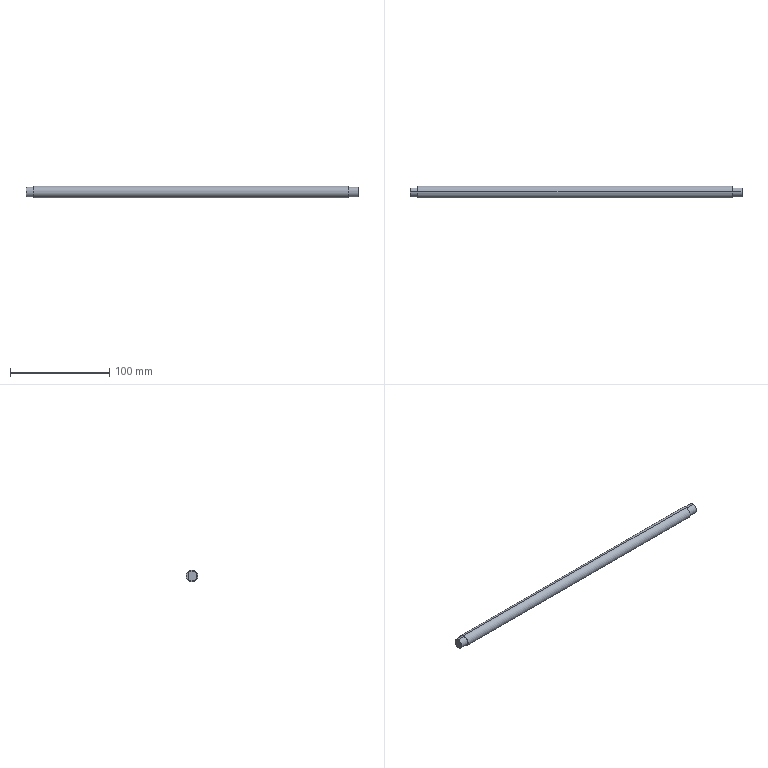Part | STEP file | 04-01 Φ12 chrome-plated rod | 1 solid | 14 faces | box 335 x 12 x 12 mm | volume 37192 mm3 | cylinder 8 | plane 6 | commonest cylinder face diameters 10 x6 12 x2
STEP:
#1=CARTESIAN_POINT('',(0.,0.,0.));
#2=DIRECTION('',(0.,0.,1.));
#3=DIRECTION('',(1.,0.,0.));
#4=AXIS2_PLACEMENT_3D('',#1,#2,#3);
#5=CARTESIAN_POINT('',(325.,0.,5.));
#6=VERTEX_POINT('',#5);
#7=CARTESIAN_POINT('',(325.,4.,3.));
#8=VERTEX_POINT('',#7);
#9=CARTESIAN_POINT('',(325.,0.,0.));
#10=DIRECTION('',(-1.,0.,0.));
#11=DIRECTION('',(0.,0.,-1.));
#12=AXIS2_PLACEMENT_3D('',#9,#10,#11);
#13=CIRCLE('',#12,5.);
#14=CARTESIAN_POINT('',(325.,0.,0.));
#15=DIRECTION('',(1.,0.,0.));
#16=DIRECTION('',(0.,0.,-1.));
#17=AXIS2_PLACEMENT_3D('',#14,#15,#16);
#18=CYLINDRICAL_SURFACE('',#17,5.);
#19=CARTESIAN_POINT('',(6.283,0.));
#20=DIRECTION('',(-1.,0.));
#21=VECTOR('',#20,1.);
#22=LINE('',#19,#21);
#23=(GEOMETRIC_REPRESENTATION_CONTEXT(2)PARAMETRIC_REPRESENTATION_CONTEXT()REPRESENTATION_CONTEXT('',''));
#24=DEFINITIONAL_REPRESENTATION('',(#22),#23);
#25=PCURVE('',#18,#24);
#26=CARTESIAN_POINT('',(325.,-6.072,6.072));
#27=DIRECTION('',(1.,0.,0.));
#28=DIRECTION('',(0.,0.,-1.));
#29=AXIS2_PLACEMENT_3D('',#26,#27,#28);
#30=PLANE('',#29);
#31=CARTESIAN_POINT('',(11.072,6.072));
#32=CARTESIAN_POINT('',(11.072,-2.588));
#33=CARTESIAN_POINT('',(3.572,1.742));
#34=CARTESIAN_POINT('',(-3.928,6.072));
#35=CARTESIAN_POINT('',(3.572,10.402));
#36=CARTESIAN_POINT('',(11.072,14.732));
#37=CARTESIAN_POINT('',(11.072,6.072));
#38=(BOUNDED_CURVE()B_SPLINE_CURVE(2,(#31,#32,#33,#34,#35,#36,#37),.UNSPECIFIED.,.T.,.F.)B_SPLINE_CURVE_WITH_KNOTS((1,2,2,2,2,1),(-2.094,0.,2.094,4.189,6.283,8.378),.UNSPECIFIED.)CURVE()GEOMETRIC_REPRESENTATION_ITEM()RATIONAL_B_SPLINE_CURVE((1.,0.5,1.,0.5,1.,0.5,1.))REPRESENTATION_ITEM(''));
#39=(GEOMETRIC_REPRESENTATION_CONTEXT(2)PARAMETRIC_REPRESENTATION_CONTEXT()REPRESENTATION_CONTEXT('',''));
#40=DEFINITIONAL_REPRESENTATION('',(#38),#39);
#41=PCURVE('',#30,#40);
#42=SURFACE_CURVE('',#13,(#25,#41),.PCURVE_S1.);
#43=EDGE_CURVE('',#6,#8,#42,.T.);
#44=ORIENTED_EDGE('',*,*,#43,.F.);
#45=CARTESIAN_POINT('',(335.,0.,5.));
#46=VERTEX_POINT('',#45);
#47=CARTESIAN_POINT('',(325.,0.,5.));
#48=DIRECTION('',(1.,0.,0.));
#49=VECTOR('',#48,1.);
#50=LINE('',#47,#49);
#51=CARTESIAN_POINT('',(3.142,0.));
#52=DIRECTION('',(0.,1.));
#53=VECTOR('',#52,1.);
#54=LINE('',#51,#53);
#55=(GEOMETRIC_REPRESENTATION_CONTEXT(2)PARAMETRIC_REPRESENTATION_CONTEXT()REPRESENTATION_CONTEXT('',''));
#56=DEFINITIONAL_REPRESENTATION('',(#54),#55);
#57=PCURVE('',#18,#56);
#58=CARTESIAN_POINT('',(325.,0.,0.));
#59=DIRECTION('',(1.,0.,0.));
#60=DIRECTION('',(0.,0.,-1.));
#61=AXIS2_PLACEMENT_3D('',#58,#59,#60);
#62=CYLINDRICAL_SURFACE('',#61,5.);
#63=CARTESIAN_POINT('',(3.142,0.));
#64=DIRECTION('',(0.,1.));
#65=VECTOR('',#64,1.);
#66=LINE('',#63,#65);
#67=(GEOMETRIC_REPRESENTATION_CONTEXT(2)PARAMETRIC_REPRESENTATION_CONTEXT()REPRESENTATION_CONTEXT('',''));
#68=DEFINITIONAL_REPRESENTATION('',(#66),#67);
#69=PCURVE('',#62,#68);
#70=SURFACE_CURVE('',#50,(#57,#69),.PCURVE_S1.);
#71=EDGE_CURVE('',#6,#46,#70,.T.);
#72=ORIENTED_EDGE('',*,*,#71,.T.);
#73=CARTESIAN_POINT('',(335.,4.,3.));
#74=VERTEX_POINT('',#73);
#75=CARTESIAN_POINT('',(335.,0.,0.));
#76=DIRECTION('',(1.,0.,0.));
#77=DIRECTION('',(0.,0.,-1.));
#78=AXIS2_PLACEMENT_3D('',#75,#76,#77);
#79=CIRCLE('',#78,5.);
#80=CARTESIAN_POINT('',(0.,10.));
#81=DIRECTION('',(1.,0.));
#82=VECTOR('',#81,1.);
#83=LINE('',#80,#82);
#84=(GEOMETRIC_REPRESENTATION_CONTEXT(2)PARAMETRIC_REPRESENTATION_CONTEXT()REPRESENTATION_CONTEXT('',''));
#85=DEFINITIONAL_REPRESENTATION('',(#83),#84);
#86=PCURVE('',#18,#85);
#87=CARTESIAN_POINT('',(335.,-5.054,5.06));
#88=DIRECTION('',(1.,0.,0.));
#89=DIRECTION('',(0.,0.,-1.));
#90=AXIS2_PLACEMENT_3D('',#87,#88,#89);
#91=PLANE('',#90);
#92=CARTESIAN_POINT('',(5.06,5.054));
#93=DIRECTION('',(1.,0.));
#94=AXIS2_PLACEMENT_2D('',#92,#93);
#95=CIRCLE('',#94,5.);
#96=(GEOMETRIC_REPRESENTATION_CONTEXT(2)PARAMETRIC_REPRESENTATION_CONTEXT()REPRESENTATION_CONTEXT('',''));
#97=DEFINITIONAL_REPRESENTATION('',(#95),#96);
#98=PCURVE('',#91,#97);
#99=SURFACE_CURVE('',#79,(#86,#98),.PCURVE_S1.);
#100=EDGE_CURVE('',#74,#46,#99,.T.);
#101=ORIENTED_EDGE('',*,*,#100,.F.);
#102=CARTESIAN_POINT('',(330.,4.,3.));
#103=DIRECTION('',(1.,0.,0.));
#104=VECTOR('',#103,1.);
#105=LINE('',#102,#104);
#106=CARTESIAN_POINT('',(2.214,5.));
#107=DIRECTION('',(0.,1.));
#108=VECTOR('',#107,1.);
#109=LINE('',#106,#108);
#110=(GEOMETRIC_REPRESENTATION_CONTEXT(2)PARAMETRIC_REPRESENTATION_CONTEXT()REPRESENTATION_CONTEXT('',''));
#111=DEFINITIONAL_REPRESENTATION('',(#109),#110);
#112=PCURVE('',#18,#111);
#113=CARTESIAN_POINT('',(325.,4.,-3.));
#114=DIRECTION('',(0.,1.,0.));
#115=DIRECTION('',(0.,0.,1.));
#116=AXIS2_PLACEMENT_3D('',#113,#114,#115);
#117=PLANE('',#116);
#118=CARTESIAN_POINT('',(6.,5.));
#119=DIRECTION('',(0.,1.));
#120=VECTOR('',#119,1.);
#121=LINE('',#118,#120);
#122=(GEOMETRIC_REPRESENTATION_CONTEXT(2)PARAMETRIC_REPRESENTATION_CONTEXT()REPRESENTATION_CONTEXT('',''));
#123=DEFINITIONAL_REPRESENTATION('',(#121),#122);
#124=PCURVE('',#117,#123);
#125=SURFACE_CURVE('',#105,(#112,#124),.PCURVE_S1.);
#126=EDGE_CURVE('',#8,#74,#125,.T.);
#127=ORIENTED_EDGE('',*,*,#126,.F.);
#128=EDGE_LOOP('',(#44,#72,#101,#127));
#129=FACE_BOUND('',#128,.T.);
#130=ADVANCED_FACE('',(#129),#18,.T.);
#131=ORIENTED_EDGE('',*,*,#71,.F.);
#132=CARTESIAN_POINT('',(325.,0.,-5.));
#133=VERTEX_POINT('',#132);
#134=CARTESIAN_POINT('',(325.,0.,0.));
#135=DIRECTION('',(-1.,0.,0.));
#136=DIRECTION('',(0.,0.,-1.));
#137=AXIS2_PLACEMENT_3D('',#134,#135,#136);
#138=CIRCLE('',#137,5.);
#139=CARTESIAN_POINT('',(6.283,0.));
#140=DIRECTION('',(-1.,0.));
#141=VECTOR('',#140,1.);
#142=LINE('',#139,#141);
#143=(GEOMETRIC_REPRESENTATION_CONTEXT(2)PARAMETRIC_REPRESENTATION_CONTEXT()REPRESENTATION_CONTEXT('',''));
#144=DEFINITIONAL_REPRESENTATION('',(#142),#143);
#145=PCURVE('',#62,#144);
#146=CARTESIAN_POINT('',(11.072,6.072));
#147=CARTESIAN_POINT('',(11.072,-2.588));
#148=CARTESIAN_POINT('',(3.572,1.742));
#149=CARTESIAN_POINT('',(-3.928,6.072));
#150=CARTESIAN_POINT('',(3.572,10.402));
#151=CARTESIAN_POINT('',(11.072,14.732));
#152=CARTESIAN_POINT('',(11.072,6.072));
#153=(BOUNDED_CURVE()B_SPLINE_CURVE(2,(#146,#147,#148,#149,#150,#151,#152),.UNSPECIFIED.,.T.,.F.)B_SPLINE_CURVE_WITH_KNOTS((1,2,2,2,2,1),(-2.094,0.,2.094,4.189,6.283,8.378),.UNSPECIFIED.)CURVE()GEOMETRIC_REPRESENTATION_ITEM()RATIONAL_B_SPLINE_CURVE((1.,0.5,1.,0.5,1.,0.5,1.))REPRESENTATION_ITEM(''));
#154=(GEOMETRIC_REPRESENTATION_CONTEXT(2)PARAMETRIC_REPRESENTATION_CONTEXT()REPRESENTATION_CONTEXT('',''));
#155=DEFINITIONAL_REPRESENTATION('',(#153),#154);
#156=PCURVE('',#30,#155);
#157=SURFACE_CURVE('',#138,(#145,#156),.PCURVE_S1.);
#158=EDGE_CURVE('',#133,#6,#157,.T.);
#159=ORIENTED_EDGE('',*,*,#158,.F.);
#160=CARTESIAN_POINT('',(335.,0.,-5.));
#161=VERTEX_POINT('',#160);
#162=CARTESIAN_POINT('',(325.,0.,-5.));
#163=DIRECTION('',(1.,0.,0.));
#164=VECTOR('',#163,1.);
#165=LINE('',#162,#164);
#166=CARTESIAN_POINT('',(6.283,0.));
#167=DIRECTION('',(0.,1.));
#168=VECTOR('',#167,1.);
#169=LINE('',#166,#168);
#170=(GEOMETRIC_REPRESENTATION_CONTEXT(2)PARAMETRIC_REPRESENTATION_CONTEXT()REPRESENTATION_CONTEXT('',''));
#171=DEFINITIONAL_REPRESENTATION('',(#169),#170);
#172=PCURVE('',#62,#171);
#173=CARTESIAN_POINT('',(325.,0.,0.));
#174=DIRECTION('',(1.,0.,0.));
#175=DIRECTION('',(0.,0.,-1.));
#176=AXIS2_PLACEMENT_3D('',#173,#174,#175);
#177=CYLINDRICAL_SURFACE('',#176,5.);
#178=CARTESIAN_POINT('',(0.,0.));
#179=DIRECTION('',(0.,1.));
#180=VECTOR('',#179,1.);
#181=LINE('',#178,#180);
#182=(GEOMETRIC_REPRESENTATION_CONTEXT(2)PARAMETRIC_REPRESENTATION_CONTEXT()REPRESENTATION_CONTEXT('',''));
#183=DEFINITIONAL_REPRESENTATION('',(#181),#182);
#184=PCURVE('',#177,#183);
#185=SURFACE_CURVE('',#165,(#172,#184),.PCURVE_S1.);
#186=EDGE_CURVE('',#133,#161,#185,.T.);
#187=ORIENTED_EDGE('',*,*,#186,.T.);
#188=CARTESIAN_POINT('',(335.,0.,0.));
#189=DIRECTION('',(1.,0.,0.));
#190=DIRECTION('',(0.,0.,-1.));
#191=AXIS2_PLACEMENT_3D('',#188,#189,#190);
#192=CIRCLE('',#191,5.);
#193=CARTESIAN_POINT('',(0.,10.));
#194=DIRECTION('',(1.,0.));
#195=VECTOR('',#194,1.);
#196=LINE('',#193,#195);
#197=(GEOMETRIC_REPRESENTATION_CONTEXT(2)PARAMETRIC_REPRESENTATION_CONTEXT()REPRESENTATION_CONTEXT('',''));
#198=DEFINITIONAL_REPRESENTATION('',(#196),#197);
#199=PCURVE('',#62,#198);
#200=CARTESIAN_POINT('',(5.06,5.054));
#201=DIRECTION('',(1.,0.));
#202=AXIS2_PLACEMENT_2D('',#200,#201);
#203=CIRCLE('',#202,5.);
#204=(GEOMETRIC_REPRESENTATION_CONTEXT(2)PARAMETRIC_REPRESENTATION_CONTEXT()REPRESENTATION_CONTEXT('',''));
#205=DEFINITIONAL_REPRESENTATION('',(#203),#204);
#206=PCURVE('',#91,#205);
#207=SURFACE_CURVE('',#192,(#199,#206),.PCURVE_S1.);
#208=EDGE_CURVE('',#46,#161,#207,.T.);
#209=ORIENTED_EDGE('',*,*,#208,.F.);
#210=EDGE_LOOP('',(#131,#159,#187,#209));
#211=FACE_BOUND('',#210,.T.);
#212=ADVANCED_FACE('',(#211),#62,.T.);
#213=CARTESIAN_POINT('',(325.,0.,-6.));
#214=VERTEX_POINT('',#213);
#215=CARTESIAN_POINT('',(325.,0.,6.));
#216=VERTEX_POINT('',#215);
#217=CARTESIAN_POINT('',(325.,0.,0.));
#218=DIRECTION('',(1.,0.,0.));
#219=DIRECTION('',(0.,0.,1.));
#220=AXIS2_PLACEMENT_3D('',#217,#218,#219);
#221=CIRCLE('',#220,6.);
#222=CARTESIAN_POINT('',(325.,0.,0.));
#223=DIRECTION('',(-1.,0.,0.));
#224=DIRECTION('',(0.,0.,1.));
#225=AXIS2_PLACEMENT_3D('',#222,#223,#224);
#226=CYLINDRICAL_SURFACE('',#225,6.);
#227=CARTESIAN_POINT('',(6.283,0.));
#228=DIRECTION('',(-1.,0.));
#229=VECTOR('',#228,1.);
#230=LINE('',#227,#229);
#231=(GEOMETRIC_REPRESENTATION_CONTEXT(2)PARAMETRIC_REPRESENTATION_CONTEXT()REPRESENTATION_CONTEXT('',''));
#232=DEFINITIONAL_REPRESENTATION('',(#230),#231);
#233=PCURVE('',#226,#232);
#234=CARTESIAN_POINT('',(6.072,6.072));
#235=DIRECTION('',(-1.,0.));
#236=AXIS2_PLACEMENT_2D('',#234,#235);
#237=CIRCLE('',#236,6.);
#238=(GEOMETRIC_REPRESENTATION_CONTEXT(2)PARAMETRIC_REPRESENTATION_CONTEXT()REPRESENTATION_CONTEXT('',''));
#239=DEFINITIONAL_REPRESENTATION('',(#237),#238);
#240=PCURVE('',#30,#239);
#241=SURFACE_CURVE('',#221,(#233,#240),.PCURVE_S1.);
#242=EDGE_CURVE('',#214,#216,#241,.T.);
#243=ORIENTED_EDGE('',*,*,#242,.F.);
#244=CARTESIAN_POINT('',(8.,0.,-6.));
#245=VERTEX_POINT('',#244);
#246=CARTESIAN_POINT('',(325.,0.,-6.));
#247=DIRECTION('',(-1.,0.,0.));
#248=VECTOR('',#247,1.);
#249=LINE('',#246,#248);
#250=CARTESIAN_POINT('',(3.142,0.));
#251=DIRECTION('',(0.,1.));
#252=VECTOR('',#251,1.);
#253=LINE('',#250,#252);
#254=(GEOMETRIC_REPRESENTATION_CONTEXT(2)PARAMETRIC_REPRESENTATION_CONTEXT()REPRESENTATION_CONTEXT('',''));
#255=DEFINITIONAL_REPRESENTATION('',(#253),#254);
#256=PCURVE('',#226,#255);
#257=CARTESIAN_POINT('',(325.,0.,0.));
#258=DIRECTION('',(-1.,0.,0.));
#259=DIRECTION('',(0.,0.,1.));
#260=AXIS2_PLACEMENT_3D('',#257,#258,#259);
#261=CYLINDRICAL_SURFACE('',#260,6.);
#262=CARTESIAN_POINT('',(3.142,0.));
#263=DIRECTION('',(0.,1.));
#264=VECTOR('',#263,1.);
#265=LINE('',#262,#264);
#266=(GEOMETRIC_REPRESENTATION_CONTEXT(2)PARAMETRIC_REPRESENTATION_CONTEXT()REPRESENTATION_CONTEXT('',''));
#267=DEFINITIONAL_REPRESENTATION('',(#265),#266);
#268=PCURVE('',#261,#267);
#269=SURFACE_CURVE('',#249,(#256,#268),.PCURVE_S1.);
#270=EDGE_CURVE('',#214,#245,#269,.T.);
#271=ORIENTED_EDGE('',*,*,#270,.T.);
#272=CARTESIAN_POINT('',(8.,0.,6.));
#273=VERTEX_POINT('',#272);
#274=CARTESIAN_POINT('',(8.,0.,0.));
#275=DIRECTION('',(-1.,0.,0.));
#276=DIRECTION('',(0.,0.,1.));
#277=AXIS2_PLACEMENT_3D('',#274,#275,#276);
#278=CIRCLE('',#277,6.);
#279=CARTESIAN_POINT('',(0.,317.));
#280=DIRECTION('',(1.,0.));
#281=VECTOR('',#280,1.);
#282=LINE('',#279,#281);
#283=(GEOMETRIC_REPRESENTATION_CONTEXT(2)PARAMETRIC_REPRESENTATION_CONTEXT()REPRESENTATION_CONTEXT('',''));
#284=DEFINITIONAL_REPRESENTATION('',(#282),#283);
#285=PCURVE('',#226,#284);
#286=CARTESIAN_POINT('',(8.,-6.072,-6.072));
#287=DIRECTION('',(-1.,0.,0.));
#288=DIRECTION('',(0.,0.,1.));
#289=AXIS2_PLACEMENT_3D('',#286,#287,#288);
#290=PLANE('',#289);
#291=CARTESIAN_POINT('',(6.072,6.072));
#292=DIRECTION('',(1.,0.));
#293=AXIS2_PLACEMENT_2D('',#291,#292);
#294=CIRCLE('',#293,6.);
#295=(GEOMETRIC_REPRESENTATION_CONTEXT(2)PARAMETRIC_REPRESENTATION_CONTEXT()REPRESENTATION_CONTEXT('',''));
#296=DEFINITIONAL_REPRESENTATION('',(#294),#295);
#297=PCURVE('',#290,#296);
#298=SURFACE_CURVE('',#278,(#285,#297),.PCURVE_S1.);
#299=EDGE_CURVE('',#273,#245,#298,.T.);
#300=ORIENTED_EDGE('',*,*,#299,.F.);
#301=CARTESIAN_POINT('',(325.,0.,6.));
#302=DIRECTION('',(-1.,0.,0.));
#303=VECTOR('',#302,1.);
#304=LINE('',#301,#303);
#305=CARTESIAN_POINT('',(0.,0.));
#306=DIRECTION('',(0.,1.));
#307=VECTOR('',#306,1.);
#308=LINE('',#305,#307);
#309=(GEOMETRIC_REPRESENTATION_CONTEXT(2)PARAMETRIC_REPRESENTATION_CONTEXT()REPRESENTATION_CONTEXT('',''));
#310=DEFINITIONAL_REPRESENTATION('',(#308),#309);
#311=PCURVE('',#226,#310);
#312=CARTESIAN_POINT('',(6.283,0.));
#313=DIRECTION('',(0.,1.));
#314=VECTOR('',#313,1.);
#315=LINE('',#312,#314);
#316=(GEOMETRIC_REPRESENTATION_CONTEXT(2)PARAMETRIC_REPRESENTATION_CONTEXT()REPRESENTATION_CONTEXT('',''));
#317=DEFINITIONAL_REPRESENTATION('',(#315),#316);
#318=PCURVE('',#261,#317);
#319=SURFACE_CURVE('',#304,(#311,#318),.PCURVE_S1.);
#320=EDGE_CURVE('',#216,#273,#319,.T.);
#321=ORIENTED_EDGE('',*,*,#320,.F.);
#322=EDGE_LOOP('',(#243,#271,#300,#321));
#323=FACE_BOUND('',#322,.T.);
#324=ADVANCED_FACE('',(#323),#226,.T.);
#325=CARTESIAN_POINT('',(8.,0.,-5.));
#326=VERTEX_POINT('',#325);
#327=CARTESIAN_POINT('',(8.,4.,-3.));
#328=VERTEX_POINT('',#327);
#329=CARTESIAN_POINT('',(8.,0.,0.));
#330=DIRECTION('',(1.,0.,0.));
#331=DIRECTION('',(0.,0.,1.));
#332=AXIS2_PLACEMENT_3D('',#329,#330,#331);
#333=CIRCLE('',#332,5.);
#334=CARTESIAN_POINT('',(8.,0.,0.));
#335=DIRECTION('',(-1.,0.,0.));
#336=DIRECTION('',(0.,0.,1.));
#337=AXIS2_PLACEMENT_3D('',#334,#335,#336);
#338=CYLINDRICAL_SURFACE('',#337,5.);
#339=CARTESIAN_POINT('',(6.283,0.));
#340=DIRECTION('',(-1.,0.));
#341=VECTOR('',#340,1.);
#342=LINE('',#339,#341);
#343=(GEOMETRIC_REPRESENTATION_CONTEXT(2)PARAMETRIC_REPRESENTATION_CONTEXT()REPRESENTATION_CONTEXT('',''));
#344=DEFINITIONAL_REPRESENTATION('',(#342),#343);
#345=PCURVE('',#338,#344);
#346=CARTESIAN_POINT('',(11.072,6.072));
#347=CARTESIAN_POINT('',(11.072,-2.588));
#348=CARTESIAN_POINT('',(3.572,1.742));
#349=CARTESIAN_POINT('',(-3.928,6.072));
#350=CARTESIAN_POINT('',(3.572,10.402));
#351=CARTESIAN_POINT('',(11.072,14.732));
#352=CARTESIAN_POINT('',(11.072,6.072));
#353=(BOUNDED_CURVE()B_SPLINE_CURVE(2,(#346,#347,#348,#349,#350,#351,#352),.UNSPECIFIED.,.T.,.F.)B_SPLINE_CURVE_WITH_KNOTS((1,2,2,2,2,1),(-2.094,0.,2.094,4.189,6.283,8.378),.UNSPECIFIED.)CURVE()GEOMETRIC_REPRESENTATION_ITEM()RATIONAL_B_SPLINE_CURVE((1.,0.5,1.,0.5,1.,0.5,1.))REPRESENTATION_ITEM(''));
#354=(GEOMETRIC_REPRESENTATION_CONTEXT(2)PARAMETRIC_REPRESENTATION_CONTEXT()REPRESENTATION_CONTEXT('',''));
#355=DEFINITIONAL_REPRESENTATION('',(#353),#354);
#356=PCURVE('',#290,#355);
#357=SURFACE_CURVE('',#333,(#345,#356),.PCURVE_S1.);
#358=EDGE_CURVE('',#326,#328,#357,.T.);
#359=ORIENTED_EDGE('',*,*,#358,.F.);
#360=CARTESIAN_POINT('',(0.,0.,-5.));
#361=VERTEX_POINT('',#360);
#362=CARTESIAN_POINT('',(8.,0.,-5.));
#363=DIRECTION('',(-1.,0.,0.));
#364=VECTOR('',#363,1.);
#365=LINE('',#362,#364);
#366=CARTESIAN_POINT('',(3.142,0.));
#367=DIRECTION('',(0.,1.));
#368=VECTOR('',#367,1.);
#369=LINE('',#366,#368);
#370=(GEOMETRIC_REPRESENTATION_CONTEXT(2)PARAMETRIC_REPRESENTATION_CONTEXT()REPRESENTATION_CONTEXT('',''));
#371=DEFINITIONAL_REPRESENTATION('',(#369),#370);
#372=PCURVE('',#338,#371);
#373=CARTESIAN_POINT('',(8.,0.,0.));
#374=DIRECTION('',(-1.,0.,0.));
#375=DIRECTION('',(0.,0.,1.));
#376=AXIS2_PLACEMENT_3D('',#373,#374,#375);
#377=CYLINDRICAL_SURFACE('',#376,5.);
#378=CARTESIAN_POINT('',(3.142,0.));
#379=DIRECTION('',(0.,1.));
#380=VECTOR('',#379,1.);
#381=LINE('',#378,#380);
#382=(GEOMETRIC_REPRESENTATION_CONTEXT(2)PARAMETRIC_REPRESENTATION_CONTEXT()REPRESENTATION_CONTEXT('',''));
#383=DEFINITIONAL_REPRESENTATION('',(#381),#382);
#384=PCURVE('',#377,#383);
#385=SURFACE_CURVE('',#365,(#372,#384),.PCURVE_S1.);
#386=EDGE_CURVE('',#326,#361,#385,.T.);
#387=ORIENTED_EDGE('',*,*,#386,.T.);
#388=CARTESIAN_POINT('',(0.,4.,-3.));
#389=VERTEX_POINT('',#388);
#390=CARTESIAN_POINT('',(0.,0.,0.));
#391=DIRECTION('',(-1.,0.,0.));
#392=DIRECTION('',(0.,0.,1.));
#393=AXIS2_PLACEMENT_3D('',#390,#391,#392);
#394=CIRCLE('',#393,5.);
#395=CARTESIAN_POINT('',(0.,8.));
#396=DIRECTION('',(1.,0.));
#397=VECTOR('',#396,1.);
#398=LINE('',#395,#397);
#399=(GEOMETRIC_REPRESENTATION_CONTEXT(2)PARAMETRIC_REPRESENTATION_CONTEXT()REPRESENTATION_CONTEXT('',''));
#400=DEFINITIONAL_REPRESENTATION('',(#398),#399);
#401=PCURVE('',#338,#400);
#402=CARTESIAN_POINT('',(0.,-5.054,5.06));
#403=DIRECTION('',(1.,0.,0.));
#404=DIRECTION('',(0.,0.,-1.));
#405=AXIS2_PLACEMENT_3D('',#402,#403,#404);
#406=PLANE('',#405);
#407=CARTESIAN_POINT('',(0.06,5.054));
#408=CARTESIAN_POINT('',(0.06,13.714));
#409=CARTESIAN_POINT('',(7.56,9.384));
#410=CARTESIAN_POINT('',(15.06,5.054));
#411=CARTESIAN_POINT('',(7.56,0.7239));
#412=CARTESIAN_POINT('',(0.06,-3.606));
#413=CARTESIAN_POINT('',(0.06,5.054));
#414=(BOUNDED_CURVE()B_SPLINE_CURVE(2,(#407,#408,#409,#410,#411,#412,#413),.UNSPECIFIED.,.T.,.F.)B_SPLINE_CURVE_WITH_KNOTS((1,2,2,2,2,1),(-2.094,0.,2.094,4.189,6.283,8.378),.UNSPECIFIED.)CURVE()GEOMETRIC_REPRESENTATION_ITEM()RATIONAL_B_SPLINE_CURVE((1.,0.5,1.,0.5,1.,0.5,1.))REPRESENTATION_ITEM(''));
#415=(GEOMETRIC_REPRESENTATION_CONTEXT(2)PARAMETRIC_REPRESENTATION_CONTEXT()REPRESENTATION_CONTEXT('',''));
#416=DEFINITIONAL_REPRESENTATION('',(#414),#415);
#417=PCURVE('',#406,#416);
#418=SURFACE_CURVE('',#394,(#401,#417),.PCURVE_S1.);
#419=EDGE_CURVE('',#389,#361,#418,.T.);
#420=ORIENTED_EDGE('',*,*,#419,.F.);
#421=CARTESIAN_POINT('',(4.,4.,-3.));
#422=DIRECTION('',(1.,0.,0.));
#423=VECTOR('',#422,1.);
#424=LINE('',#421,#423);
#425=CARTESIAN_POINT('',(2.214,4.));
#426=DIRECTION('',(0.,-1.));
#427=VECTOR('',#426,1.);
#428=LINE('',#425,#427);
#429=(GEOMETRIC_REPRESENTATION_CONTEXT(2)PARAMETRIC_REPRESENTATION_CONTEXT()REPRESENTATION_CONTEXT('',''));
#430=DEFINITIONAL_REPRESENTATION('',(#428),#429);
#431=PCURVE('',#338,#430);
#432=CARTESIAN_POINT('',(0.,4.,3.));
#433=DIRECTION('',(0.,-1.,0.));
#434=DIRECTION('',(0.,0.,-1.));
#435=AXIS2_PLACEMENT_3D('',#432,#433,#434);
#436=PLANE('',#435);
#437=CARTESIAN_POINT('',(6.,4.));
#438=DIRECTION('',(0.,1.));
#439=VECTOR('',#438,1.);
#440=LINE('',#437,#439);
#441=(GEOMETRIC_REPRESENTATION_CONTEXT(2)PARAMETRIC_REPRESENTATION_CONTEXT()REPRESENTATION_CONTEXT('',''));
#442=DEFINITIONAL_REPRESENTATION('',(#440),#441);
#443=PCURVE('',#436,#442);
#444=SURFACE_CURVE('',#424,(#431,#443),.PCURVE_S1.);
#445=EDGE_CURVE('',#389,#328,#444,.T.);
#446=ORIENTED_EDGE('',*,*,#445,.T.);
#447=EDGE_LOOP('',(#359,#387,#420,#446));
#448=FACE_BOUND('',#447,.T.);
#449=ADVANCED_FACE('',(#448),#338,.T.);
#450=ORIENTED_EDGE('',*,*,#386,.F.);
#451=CARTESIAN_POINT('',(8.,0.,5.));
#452=VERTEX_POINT('',#451);
#453=CARTESIAN_POINT('',(8.,0.,0.));
#454=DIRECTION('',(1.,0.,0.));
#455=DIRECTION('',(0.,0.,1.));
#456=AXIS2_PLACEMENT_3D('',#453,#454,#455);
#457=CIRCLE('',#456,5.);
#458=CARTESIAN_POINT('',(6.283,0.));
#459=DIRECTION('',(-1.,0.));
#460=VECTOR('',#459,1.);
#461=LINE('',#458,#460);
#462=(GEOMETRIC_REPRESENTATION_CONTEXT(2)PARAMETRIC_REPRESENTATION_CONTEXT()REPRESENTATION_CONTEXT('',''));
#463=DEFINITIONAL_REPRESENTATION('',(#461),#462);
#464=PCURVE('',#377,#463);
#465=CARTESIAN_POINT('',(11.072,6.072));
#466=CARTESIAN_POINT('',(11.072,-2.588));
#467=CARTESIAN_POINT('',(3.572,1.742));
#468=CARTESIAN_POINT('',(-3.928,6.072));
#469=CARTESIAN_POINT('',(3.572,10.402));
#470=CARTESIAN_POINT('',(11.072,14.732));
#471=CARTESIAN_POINT('',(11.072,6.072));
#472=(BOUNDED_CURVE()B_SPLINE_CURVE(2,(#465,#466,#467,#468,#469,#470,#471),.UNSPECIFIED.,.T.,.F.)B_SPLINE_CURVE_WITH_KNOTS((1,2,2,2,2,1),(-2.094,0.,2.094,4.189,6.283,8.378),.UNSPECIFIED.)CURVE()GEOMETRIC_REPRESENTATION_ITEM()RATIONAL_B_SPLINE_CURVE((1.,0.5,1.,0.5,1.,0.5,1.))REPRESENTATION_ITEM(''));
#473=(GEOMETRIC_REPRESENTATION_CONTEXT(2)PARAMETRIC_REPRESENTATION_CONTEXT()REPRESENTATION_CONTEXT('',''));
#474=DEFINITIONAL_REPRESENTATION('',(#472),#473);
#475=PCURVE('',#290,#474);
#476=SURFACE_CURVE('',#457,(#464,#475),.PCURVE_S1.);
#477=EDGE_CURVE('',#452,#326,#476,.T.);
#478=ORIENTED_EDGE('',*,*,#477,.F.);
#479=CARTESIAN_POINT('',(0.,0.,5.));
#480=VERTEX_POINT('',#479);
#481=CARTESIAN_POINT('',(8.,0.,5.));
#482=DIRECTION('',(-1.,0.,0.));
#483=VECTOR('',#482,1.);
#484=LINE('',#481,#483);
#485=CARTESIAN_POINT('',(6.283,0.));
#486=DIRECTION('',(0.,1.));
#487=VECTOR('',#486,1.);
#488=LINE('',#485,#487);
#489=(GEOMETRIC_REPRESENTATION_CONTEXT(2)PARAMETRIC_REPRESENTATION_CONTEXT()REPRESENTATION_CONTEXT('',''));
#490=DEFINITIONAL_REPRESENTATION('',(#488),#489);
#491=PCURVE('',#377,#490);
#492=CARTESIAN_POINT('',(8.,0.,0.));
#493=DIRECTION('',(-1.,0.,0.));
#494=DIRECTION('',(0.,0.,1.));
#495=AXIS2_PLACEMENT_3D('',#492,#493,#494);
#496=CYLINDRICAL_SURFACE('',#495,5.);
#497=CARTESIAN_POINT('',(0.,0.));
#498=DIRECTION('',(0.,1.));
#499=VECTOR('',#498,1.);
#500=LINE('',#497,#499);
#501=(GEOMETRIC_REPRESENTATION_CONTEXT(2)PARAMETRIC_REPRESENTATION_CONTEXT()REPRESENTATION_CONTEXT('',''));
#502=DEFINITIONAL_REPRESENTATION('',(#500),#501);
#503=PCURVE('',#496,#502);
#504=SURFACE_CURVE('',#484,(#491,#503),.PCURVE_S1.);
#505=EDGE_CURVE('',#452,#480,#504,.T.);
#506=ORIENTED_EDGE('',*,*,#505,.T.);
#507=CARTESIAN_POINT('',(0.,0.,0.));
#508=DIRECTION('',(-1.,0.,0.));
#509=DIRECTION('',(0.,0.,1.));
#510=AXIS2_PLACEMENT_3D('',#507,#508,#509);
#511=CIRCLE('',#510,5.);
#512=CARTESIAN_POINT('',(0.,8.));
#513=DIRECTION('',(1.,0.));
#514=VECTOR('',#513,1.);
#515=LINE('',#512,#514);
#516=(GEOMETRIC_REPRESENTATION_CONTEXT(2)PARAMETRIC_REPRESENTATION_CONTEXT()REPRESENTATION_CONTEXT('',''));
#517=DEFINITIONAL_REPRESENTATION('',(#515),#516);
#518=PCURVE('',#377,#517);
#519=CARTESIAN_POINT('',(0.06,5.054));
#520=CARTESIAN_POINT('',(0.06,13.714));
#521=CARTESIAN_POINT('',(7.56,9.384));
#522=CARTESIAN_POINT('',(15.06,5.054));
#523=CARTESIAN_POINT('',(7.56,0.7239));
#524=CARTESIAN_POINT('',(0.06,-3.606));
#525=CARTESIAN_POINT('',(0.06,5.054));
#526=(BOUNDED_CURVE()B_SPLINE_CURVE(2,(#519,#520,#521,#522,#523,#524,#525),.UNSPECIFIED.,.T.,.F.)B_SPLINE_CURVE_WITH_KNOTS((1,2,2,2,2,1),(-2.094,0.,2.094,4.189,6.283,8.378),.UNSPECIFIED.)CURVE()GEOMETRIC_REPRESENTATION_ITEM()RATIONAL_B_SPLINE_CURVE((1.,0.5,1.,0.5,1.,0.5,1.))REPRESENTATION_ITEM(''));
#527=(GEOMETRIC_REPRESENTATION_CONTEXT(2)PARAMETRIC_REPRESENTATION_CONTEXT()REPRESENTATION_CONTEXT('',''));
#528=DEFINITIONAL_REPRESENTATION('',(#526),#527);
#529=PCURVE('',#406,#528);
#530=SURFACE_CURVE('',#511,(#518,#529),.PCURVE_S1.);
#531=EDGE_CURVE('',#361,#480,#530,.T.);
#532=ORIENTED_EDGE('',*,*,#531,.F.);
#533=EDGE_LOOP('',(#450,#478,#506,#532));
#534=FACE_BOUND('',#533,.T.);
#535=ADVANCED_FACE('',(#534),#377,.T.);
#536=ORIENTED_EDGE('',*,*,#186,.F.);
#537=CARTESIAN_POINT('',(325.,4.,-3.));
#538=VERTEX_POINT('',#537);
#539=CARTESIAN_POINT('',(325.,0.,0.));
#540=DIRECTION('',(-1.,0.,0.));
#541=DIRECTION('',(0.,0.,-1.));
#542=AXIS2_PLACEMENT_3D('',#539,#540,#541);
#543=CIRCLE('',#542,5.);
#544=CARTESIAN_POINT('',(6.283,0.));
#545=DIRECTION('',(-1.,0.));
#546=VECTOR('',#545,1.);
#547=LINE('',#544,#546);
#548=(GEOMETRIC_REPRESENTATION_CONTEXT(2)PARAMETRIC_REPRESENTATION_CONTEXT()REPRESENTATION_CONTEXT('',''));
#549=DEFINITIONAL_REPRESENTATION('',(#547),#548);
#550=PCURVE('',#177,#549);
#551=CARTESIAN_POINT('',(11.072,6.072));
#552=CARTESIAN_POINT('',(11.072,-2.588));
#553=CARTESIAN_POINT('',(3.572,1.742));
#554=CARTESIAN_POINT('',(-3.928,6.072));
#555=CARTESIAN_POINT('',(3.572,10.402));
#556=CARTESIAN_POINT('',(11.072,14.732));
#557=CARTESIAN_POINT('',(11.072,6.072));
#558=(BOUNDED_CURVE()B_SPLINE_CURVE(2,(#551,#552,#553,#554,#555,#556,#557),.UNSPECIFIED.,.T.,.F.)B_SPLINE_CURVE_WITH_KNOTS((1,2,2,2,2,1),(-2.094,0.,2.094,4.189,6.283,8.378),.UNSPECIFIED.)CURVE()GEOMETRIC_REPRESENTATION_ITEM()RATIONAL_B_SPLINE_CURVE((1.,0.5,1.,0.5,1.,0.5,1.))REPRESENTATION_ITEM(''));
#559=(GEOMETRIC_REPRESENTATION_CONTEXT(2)PARAMETRIC_REPRESENTATION_CONTEXT()REPRESENTATION_CONTEXT('',''));
#560=DEFINITIONAL_REPRESENTATION('',(#558),#559);
#561=PCURVE('',#30,#560);
#562=SURFACE_CURVE('',#543,(#550,#561),.PCURVE_S1.);
#563=EDGE_CURVE('',#538,#133,#562,.T.);
#564=ORIENTED_EDGE('',*,*,#563,.F.);
#565=CARTESIAN_POINT('',(335.,4.,-3.));
#566=VERTEX_POINT('',#565);
#567=CARTESIAN_POINT('',(330.,4.,-3.));
#568=DIRECTION('',(-1.,0.,0.));
#569=VECTOR('',#568,1.);
#570=LINE('',#567,#569);
#571=CARTESIAN_POINT('',(0.9273,5.));
#572=DIRECTION('',(0.,-1.));
#573=VECTOR('',#572,1.);
#574=LINE('',#571,#573);
#575=(GEOMETRIC_REPRESENTATION_CONTEXT(2)PARAMETRIC_REPRESENTATION_CONTEXT()REPRESENTATION_CONTEXT('',''));
#576=DEFINITIONAL_REPRESENTATION('',(#574),#575);
#577=PCURVE('',#177,#576);
#578=CARTESIAN_POINT('',(0.,5.));
#579=DIRECTION('',(0.,-1.));
#580=VECTOR('',#579,1.);
#581=LINE('',#578,#580);
#582=(GEOMETRIC_REPRESENTATION_CONTEXT(2)PARAMETRIC_REPRESENTATION_CONTEXT()REPRESENTATION_CONTEXT('',''));
#583=DEFINITIONAL_REPRESENTATION('',(#581),#582);
#584=PCURVE('',#117,#583);
#585=SURFACE_CURVE('',#570,(#577,#584),.PCURVE_S1.);
#586=EDGE_CURVE('',#566,#538,#585,.T.);
#587=ORIENTED_EDGE('',*,*,#586,.F.);
#588=CARTESIAN_POINT('',(335.,0.,0.));
#589=DIRECTION('',(1.,0.,0.));
#590=DIRECTION('',(0.,0.,-1.));
#591=AXIS2_PLACEMENT_3D('',#588,#589,#590);
#592=CIRCLE('',#591,5.);
#593=CARTESIAN_POINT('',(0.,10.));
#594=DIRECTION('',(1.,0.));
#595=VECTOR('',#594,1.);
#596=LINE('',#593,#595);
#597=(GEOMETRIC_REPRESENTATION_CONTEXT(2)PARAMETRIC_REPRESENTATION_CONTEXT()REPRESENTATION_CONTEXT('',''));
#598=DEFINITIONAL_REPRESENTATION('',(#596),#597);
#599=PCURVE('',#177,#598);
#600=CARTESIAN_POINT('',(5.06,5.054));
#601=DIRECTION('',(1.,0.));
#602=AXIS2_PLACEMENT_2D('',#600,#601);
#603=CIRCLE('',#602,5.);
#604=(GEOMETRIC_REPRESENTATION_CONTEXT(2)PARAMETRIC_REPRESENTATION_CONTEXT()REPRESENTATION_CONTEXT('',''));
#605=DEFINITIONAL_REPRESENTATION('',(#603),#604);
#606=PCURVE('',#91,#605);
#607=SURFACE_CURVE('',#592,(#599,#606),.PCURVE_S1.);
#608=EDGE_CURVE('',#161,#566,#607,.T.);
#609=ORIENTED_EDGE('',*,*,#608,.F.);
#610=EDGE_LOOP('',(#536,#564,#587,#609));
#611=FACE_BOUND('',#610,.T.);
#612=ADVANCED_FACE('',(#611),#177,.T.);
#613=CARTESIAN_POINT('',(325.,4.,0.));
#614=DIRECTION('',(0.,0.,-1.));
#615=VECTOR('',#614,1.);
#616=LINE('',#613,#615);
#617=CARTESIAN_POINT('',(6.072,10.072));
#618=DIRECTION('',(1.,0.));
#619=VECTOR('',#618,1.);
#620=LINE('',#617,#619);
#621=(GEOMETRIC_REPRESENTATION_CONTEXT(2)PARAMETRIC_REPRESENTATION_CONTEXT()REPRESENTATION_CONTEXT('',''));
#622=DEFINITIONAL_REPRESENTATION('',(#620),#621);
#623=PCURVE('',#30,#622);
#624=CARTESIAN_POINT('',(3.,0.));
#625=DIRECTION('',(-1.,0.));
#626=VECTOR('',#625,1.);
#627=LINE('',#624,#626);
#628=(GEOMETRIC_REPRESENTATION_CONTEXT(2)PARAMETRIC_REPRESENTATION_CONTEXT()REPRESENTATION_CONTEXT('',''));
#629=DEFINITIONAL_REPRESENTATION('',(#627),#628);
#630=PCURVE('',#117,#629);
#631=SURFACE_CURVE('',#616,(#623,#630),.PCURVE_S1.);
#632=EDGE_CURVE('',#8,#538,#631,.T.);
#633=ORIENTED_EDGE('',*,*,#632,.T.);
#634=ORIENTED_EDGE('',*,*,#563,.T.);
#635=ORIENTED_EDGE('',*,*,#158,.T.);
#636=ORIENTED_EDGE('',*,*,#43,.T.);
#637=EDGE_LOOP('',(#633,#634,#635,#636));
#638=FACE_BOUND('',#637,.T.);
#639=CARTESIAN_POINT('',(325.,0.,0.));
#640=DIRECTION('',(1.,0.,0.));
#641=DIRECTION('',(0.,0.,1.));
#642=AXIS2_PLACEMENT_3D('',#639,#640,#641);
#643=CIRCLE('',#642,6.);
#644=CARTESIAN_POINT('',(6.072,6.072));
#645=DIRECTION('',(-1.,0.));
#646=AXIS2_PLACEMENT_2D('',#644,#645);
#647=CIRCLE('',#646,6.);
#648=(GEOMETRIC_REPRESENTATION_CONTEXT(2)PARAMETRIC_REPRESENTATION_CONTEXT()REPRESENTATION_CONTEXT('',''));
#649=DEFINITIONAL_REPRESENTATION('',(#647),#648);
#650=PCURVE('',#30,#649);
#651=CARTESIAN_POINT('',(6.283,0.));
#652=DIRECTION('',(-1.,0.));
#653=VECTOR('',#652,1.);
#654=LINE('',#651,#653);
#655=(GEOMETRIC_REPRESENTATION_CONTEXT(2)PARAMETRIC_REPRESENTATION_CONTEXT()REPRESENTATION_CONTEXT('',''));
#656=DEFINITIONAL_REPRESENTATION('',(#654),#655);
#657=PCURVE('',#261,#656);
#658=SURFACE_CURVE('',#643,(#650,#657),.PCURVE_S1.);
#659=EDGE_CURVE('',#216,#214,#658,.T.);
#660=ORIENTED_EDGE('',*,*,#659,.T.);
#661=ORIENTED_EDGE('',*,*,#242,.T.);
#662=EDGE_LOOP('',(#660,#661));
#663=FACE_BOUND('',#662,.T.);
#664=ADVANCED_FACE('',(#638,#663),#30,.T.);
#665=ORIENTED_EDGE('',*,*,#100,.T.);
#666=ORIENTED_EDGE('',*,*,#208,.T.);
#667=ORIENTED_EDGE('',*,*,#608,.T.);
#668=CARTESIAN_POINT('',(335.,4.,0.));
#669=DIRECTION('',(0.,0.,1.));
#670=VECTOR('',#669,1.);
#671=LINE('',#668,#670);
#672=CARTESIAN_POINT('',(5.06,9.054));
#673=DIRECTION('',(-1.,0.));
#674=VECTOR('',#673,1.);
#675=LINE('',#672,#674);
#676=(GEOMETRIC_REPRESENTATION_CONTEXT(2)PARAMETRIC_REPRESENTATION_CONTEXT()REPRESENTATION_CONTEXT('',''));
#677=DEFINITIONAL_REPRESENTATION('',(#675),#676);
#678=PCURVE('',#91,#677);
#679=CARTESIAN_POINT('',(3.,10.));
#680=DIRECTION('',(1.,0.));
#681=VECTOR('',#680,1.);
#682=LINE('',#679,#681);
#683=(GEOMETRIC_REPRESENTATION_CONTEXT(2)PARAMETRIC_REPRESENTATION_CONTEXT()REPRESENTATION_CONTEXT('',''));
#684=DEFINITIONAL_REPRESENTATION('',(#682),#683);
#685=PCURVE('',#117,#684);
#686=SURFACE_CURVE('',#671,(#678,#685),.PCURVE_S1.);
#687=EDGE_CURVE('',#566,#74,#686,.T.);
#688=ORIENTED_EDGE('',*,*,#687,.T.);
#689=EDGE_LOOP('',(#665,#666,#667,#688));
#690=FACE_BOUND('',#689,.T.);
#691=ADVANCED_FACE('',(#690),#91,.T.);
#692=ORIENTED_EDGE('',*,*,#586,.T.);
#693=ORIENTED_EDGE('',*,*,#632,.F.);
#694=ORIENTED_EDGE('',*,*,#126,.T.);
#695=ORIENTED_EDGE('',*,*,#687,.F.);
#696=EDGE_LOOP('',(#692,#693,#694,#695));
#697=FACE_BOUND('',#696,.T.);
#698=ADVANCED_FACE('',(#697),#117,.T.);
#699=ORIENTED_EDGE('',*,*,#270,.F.);
#700=ORIENTED_EDGE('',*,*,#659,.F.);
#701=ORIENTED_EDGE('',*,*,#320,.T.);
#702=CARTESIAN_POINT('',(8.,0.,0.));
#703=DIRECTION('',(-1.,0.,0.));
#704=DIRECTION('',(0.,0.,1.));
#705=AXIS2_PLACEMENT_3D('',#702,#703,#704);
#706=CIRCLE('',#705,6.);
#707=CARTESIAN_POINT('',(0.,317.));
#708=DIRECTION('',(1.,0.));
#709=VECTOR('',#708,1.);
#710=LINE('',#707,#709);
#711=(GEOMETRIC_REPRESENTATION_CONTEXT(2)PARAMETRIC_REPRESENTATION_CONTEXT()REPRESENTATION_CONTEXT('',''));
#712=DEFINITIONAL_REPRESENTATION('',(#710),#711);
#713=PCURVE('',#261,#712);
#714=CARTESIAN_POINT('',(6.072,6.072));
#715=DIRECTION('',(1.,0.));
#716=AXIS2_PLACEMENT_2D('',#714,#715);
#717=CIRCLE('',#716,6.);
#718=(GEOMETRIC_REPRESENTATION_CONTEXT(2)PARAMETRIC_REPRESENTATION_CONTEXT()REPRESENTATION_CONTEXT('',''));
#719=DEFINITIONAL_REPRESENTATION('',(#717),#718);
#720=PCURVE('',#290,#719);
#721=SURFACE_CURVE('',#706,(#713,#720),.PCURVE_S1.);
#722=EDGE_CURVE('',#245,#273,#721,.T.);
#723=ORIENTED_EDGE('',*,*,#722,.F.);
#724=EDGE_LOOP('',(#699,#700,#701,#723));
#725=FACE_BOUND('',#724,.T.);
#726=ADVANCED_FACE('',(#725),#261,.T.);
#727=CARTESIAN_POINT('',(8.,4.,3.));
#728=VERTEX_POINT('',#727);
#729=CARTESIAN_POINT('',(8.,4.,0.));
#730=DIRECTION('',(0.,0.,1.));
#731=VECTOR('',#730,1.);
#732=LINE('',#729,#731);
#733=CARTESIAN_POINT('',(6.072,10.072));
#734=DIRECTION('',(1.,0.));
#735=VECTOR('',#734,1.);
#736=LINE('',#733,#735);
#737=(GEOMETRIC_REPRESENTATION_CONTEXT(2)PARAMETRIC_REPRESENTATION_CONTEXT()REPRESENTATION_CONTEXT('',''));
#738=DEFINITIONAL_REPRESENTATION('',(#736),#737);
#739=PCURVE('',#290,#738);
#740=CARTESIAN_POINT('',(3.,8.));
#741=DIRECTION('',(-1.,0.));
#742=VECTOR('',#741,1.);
#743=LINE('',#740,#742);
#744=(GEOMETRIC_REPRESENTATION_CONTEXT(2)PARAMETRIC_REPRESENTATION_CONTEXT()REPRESENTATION_CONTEXT('',''));
#745=DEFINITIONAL_REPRESENTATION('',(#743),#744);
#746=PCURVE('',#436,#745);
#747=SURFACE_CURVE('',#732,(#739,#746),.PCURVE_S1.);
#748=EDGE_CURVE('',#328,#728,#747,.T.);
#749=ORIENTED_EDGE('',*,*,#748,.T.);
#750=CARTESIAN_POINT('',(8.,0.,0.));
#751=DIRECTION('',(1.,0.,0.));
#752=DIRECTION('',(0.,0.,1.));
#753=AXIS2_PLACEMENT_3D('',#750,#751,#752);
#754=CIRCLE('',#753,5.);
#755=CARTESIAN_POINT('',(11.072,6.072));
#756=CARTESIAN_POINT('',(11.072,-2.588));
#757=CARTESIAN_POINT('',(3.572,1.742));
#758=CARTESIAN_POINT('',(-3.928,6.072));
#759=CARTESIAN_POINT('',(3.572,10.402));
#760=CARTESIAN_POINT('',(11.072,14.732));
#761=CARTESIAN_POINT('',(11.072,6.072));
#762=(BOUNDED_CURVE()B_SPLINE_CURVE(2,(#755,#756,#757,#758,#759,#760,#761),.UNSPECIFIED.,.T.,.F.)B_SPLINE_CURVE_WITH_KNOTS((1,2,2,2,2,1),(-2.094,0.,2.094,4.189,6.283,8.378),.UNSPECIFIED.)CURVE()GEOMETRIC_REPRESENTATION_ITEM()RATIONAL_B_SPLINE_CURVE((1.,0.5,1.,0.5,1.,0.5,1.))REPRESENTATION_ITEM(''));
#763=(GEOMETRIC_REPRESENTATION_CONTEXT(2)PARAMETRIC_REPRESENTATION_CONTEXT()REPRESENTATION_CONTEXT('',''));
#764=DEFINITIONAL_REPRESENTATION('',(#762),#763);
#765=PCURVE('',#290,#764);
#766=CARTESIAN_POINT('',(6.283,0.));
#767=DIRECTION('',(-1.,0.));
#768=VECTOR('',#767,1.);
#769=LINE('',#766,#768);
#770=(GEOMETRIC_REPRESENTATION_CONTEXT(2)PARAMETRIC_REPRESENTATION_CONTEXT()REPRESENTATION_CONTEXT('',''));
#771=DEFINITIONAL_REPRESENTATION('',(#769),#770);
#772=PCURVE('',#496,#771);
#773=SURFACE_CURVE('',#754,(#765,#772),.PCURVE_S1.);
#774=EDGE_CURVE('',#728,#452,#773,.T.);
#775=ORIENTED_EDGE('',*,*,#774,.T.);
#776=ORIENTED_EDGE('',*,*,#477,.T.);
#777=ORIENTED_EDGE('',*,*,#358,.T.);
#778=EDGE_LOOP('',(#749,#775,#776,#777));
#779=FACE_BOUND('',#778,.T.);
#780=ORIENTED_EDGE('',*,*,#299,.T.);
#781=ORIENTED_EDGE('',*,*,#722,.T.);
#782=EDGE_LOOP('',(#780,#781));
#783=FACE_BOUND('',#782,.T.);
#784=ADVANCED_FACE('',(#779,#783),#290,.T.);
#785=ORIENTED_EDGE('',*,*,#505,.F.);
#786=ORIENTED_EDGE('',*,*,#774,.F.);
#787=CARTESIAN_POINT('',(0.,4.,3.));
#788=VERTEX_POINT('',#787);
#789=CARTESIAN_POINT('',(4.,4.,3.));
#790=DIRECTION('',(1.,0.,0.));
#791=VECTOR('',#790,1.);
#792=LINE('',#789,#791);
#793=CARTESIAN_POINT('',(0.9273,4.));
#794=DIRECTION('',(0.,-1.));
#795=VECTOR('',#794,1.);
#796=LINE('',#793,#795);
#797=(GEOMETRIC_REPRESENTATION_CONTEXT(2)PARAMETRIC_REPRESENTATION_CONTEXT()REPRESENTATION_CONTEXT('',''));
#798=DEFINITIONAL_REPRESENTATION('',(#796),#797);
#799=PCURVE('',#496,#798);
#800=CARTESIAN_POINT('',(0.,4.));
#801=DIRECTION('',(0.,1.));
#802=VECTOR('',#801,1.);
#803=LINE('',#800,#802);
#804=(GEOMETRIC_REPRESENTATION_CONTEXT(2)PARAMETRIC_REPRESENTATION_CONTEXT()REPRESENTATION_CONTEXT('',''));
#805=DEFINITIONAL_REPRESENTATION('',(#803),#804);
#806=PCURVE('',#436,#805);
#807=SURFACE_CURVE('',#792,(#799,#806),.PCURVE_S1.);
#808=EDGE_CURVE('',#788,#728,#807,.T.);
#809=ORIENTED_EDGE('',*,*,#808,.F.);
#810=CARTESIAN_POINT('',(0.,0.,0.));
#811=DIRECTION('',(-1.,0.,0.));
#812=DIRECTION('',(0.,0.,1.));
#813=AXIS2_PLACEMENT_3D('',#810,#811,#812);
#814=CIRCLE('',#813,5.);
#815=CARTESIAN_POINT('',(0.,8.));
#816=DIRECTION('',(1.,0.));
#817=VECTOR('',#816,1.);
#818=LINE('',#815,#817);
#819=(GEOMETRIC_REPRESENTATION_CONTEXT(2)PARAMETRIC_REPRESENTATION_CONTEXT()REPRESENTATION_CONTEXT('',''));
#820=DEFINITIONAL_REPRESENTATION('',(#818),#819);
#821=PCURVE('',#496,#820);
#822=CARTESIAN_POINT('',(0.06,5.054));
#823=CARTESIAN_POINT('',(0.06,13.714));
#824=CARTESIAN_POINT('',(7.56,9.384));
#825=CARTESIAN_POINT('',(15.06,5.054));
#826=CARTESIAN_POINT('',(7.56,0.7239));
#827=CARTESIAN_POINT('',(0.06,-3.606));
#828=CARTESIAN_POINT('',(0.06,5.054));
#829=(BOUNDED_CURVE()B_SPLINE_CURVE(2,(#822,#823,#824,#825,#826,#827,#828),.UNSPECIFIED.,.T.,.F.)B_SPLINE_CURVE_WITH_KNOTS((1,2,2,2,2,1),(-2.094,0.,2.094,4.189,6.283,8.378),.UNSPECIFIED.)CURVE()GEOMETRIC_REPRESENTATION_ITEM()RATIONAL_B_SPLINE_CURVE((1.,0.5,1.,0.5,1.,0.5,1.))REPRESENTATION_ITEM(''));
#830=(GEOMETRIC_REPRESENTATION_CONTEXT(2)PARAMETRIC_REPRESENTATION_CONTEXT()REPRESENTATION_CONTEXT('',''));
#831=DEFINITIONAL_REPRESENTATION('',(#829),#830);
#832=PCURVE('',#406,#831);
#833=SURFACE_CURVE('',#814,(#821,#832),.PCURVE_S1.);
#834=EDGE_CURVE('',#480,#788,#833,.T.);
#835=ORIENTED_EDGE('',*,*,#834,.F.);
#836=EDGE_LOOP('',(#785,#786,#809,#835));
#837=FACE_BOUND('',#836,.T.);
#838=ADVANCED_FACE('',(#837),#496,.T.);
#839=ORIENTED_EDGE('',*,*,#748,.F.);
#840=ORIENTED_EDGE('',*,*,#445,.F.);
#841=CARTESIAN_POINT('',(0.,4.,0.));
#842=DIRECTION('',(0.,0.,-1.));
#843=VECTOR('',#842,1.);
#844=LINE('',#841,#843);
#845=CARTESIAN_POINT('',(3.,0.));
#846=DIRECTION('',(1.,0.));
#847=VECTOR('',#846,1.);
#848=LINE('',#845,#847);
#849=(GEOMETRIC_REPRESENTATION_CONTEXT(2)PARAMETRIC_REPRESENTATION_CONTEXT()REPRESENTATION_CONTEXT('',''));
#850=DEFINITIONAL_REPRESENTATION('',(#848),#849);
#851=PCURVE('',#436,#850);
#852=CARTESIAN_POINT('',(5.06,9.054));
#853=DIRECTION('',(1.,0.));
#854=VECTOR('',#853,1.);
#855=LINE('',#852,#854);
#856=(GEOMETRIC_REPRESENTATION_CONTEXT(2)PARAMETRIC_REPRESENTATION_CONTEXT()REPRESENTATION_CONTEXT('',''));
#857=DEFINITIONAL_REPRESENTATION('',(#855),#856);
#858=PCURVE('',#406,#857);
#859=SURFACE_CURVE('',#844,(#851,#858),.PCURVE_S1.);
#860=EDGE_CURVE('',#788,#389,#859,.T.);
#861=ORIENTED_EDGE('',*,*,#860,.F.);
#862=ORIENTED_EDGE('',*,*,#808,.T.);
#863=EDGE_LOOP('',(#839,#840,#861,#862));
#864=FACE_BOUND('',#863,.T.);
#865=ADVANCED_FACE('',(#864),#436,.F.);
#866=ORIENTED_EDGE('',*,*,#419,.T.);
#867=ORIENTED_EDGE('',*,*,#531,.T.);
#868=ORIENTED_EDGE('',*,*,#834,.T.);
#869=ORIENTED_EDGE('',*,*,#860,.T.);
#870=EDGE_LOOP('',(#866,#867,#868,#869));
#871=FACE_BOUND('',#870,.T.);
#872=ADVANCED_FACE('',(#871),#406,.F.);
#873=CLOSED_SHELL('',(#130,#212,#324,#449,#535,#612,#664,#691,#698,#726,#784,#838,#865,#872));
#874=MANIFOLD_SOLID_BREP('',#873);
#875=(LENGTH_UNIT()NAMED_UNIT(*)SI_UNIT(.MILLI.,.METRE.));
#876=UNCERTAINTY_MEASURE_WITH_UNIT(LENGTH_MEASURE(0.0000001),#875,'','');
#877=(NAMED_UNIT(*)PLANE_ANGLE_UNIT()SI_UNIT($,.RADIAN.));
#878=(NAMED_UNIT(*)SI_UNIT($,.STERADIAN.)SOLID_ANGLE_UNIT());
#879=(GEOMETRIC_REPRESENTATION_CONTEXT(3)GLOBAL_UNCERTAINTY_ASSIGNED_CONTEXT((#876))GLOBAL_UNIT_ASSIGNED_CONTEXT((#875,#877,#878))REPRESENTATION_CONTEXT('',''));
#880=ADVANCED_BREP_SHAPE_REPRESENTATION('',(#4,#874),#879);